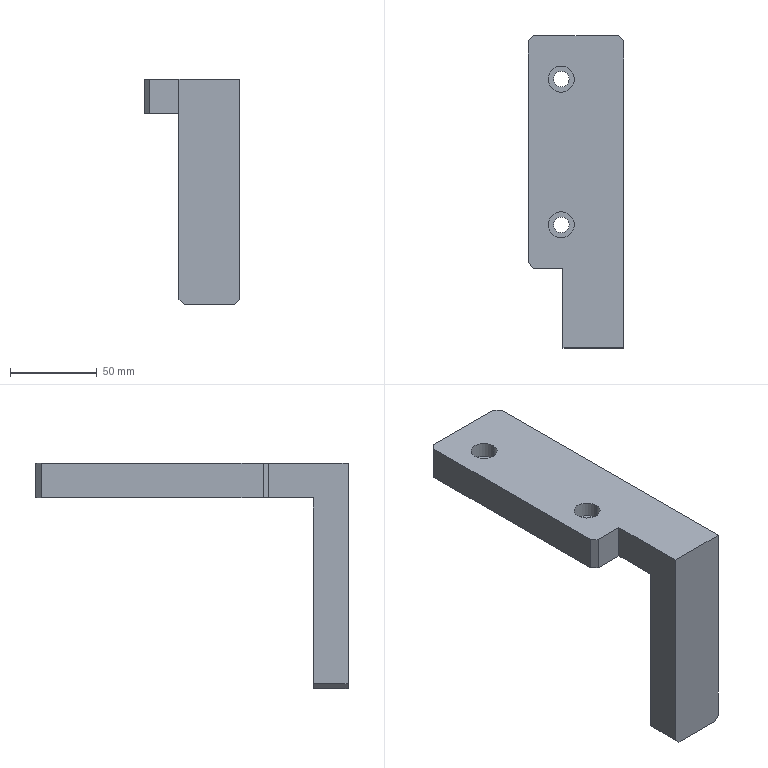Part | STEP file | 1 solid | 25 faces | box 55 x 180 x 130 mm | volume 251570 mm3 | plane 17 | cylinder 8 | commonest cylinder face diameters 9 x4 15 x4